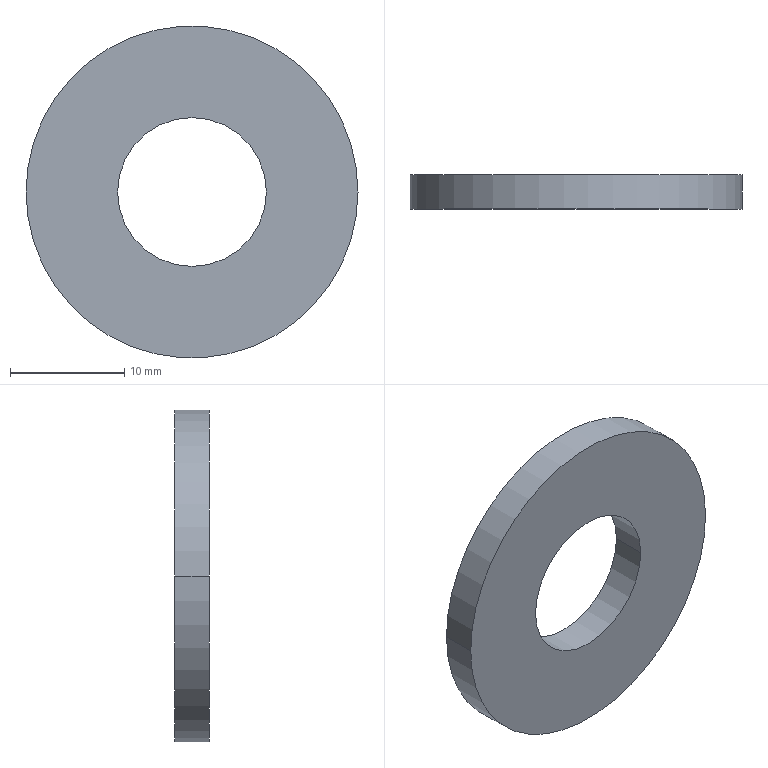Part | STEP file | LIB_29542724_CUP_SPRING_M12 | 1 solid | 6 faces | box 29 x 3 x 29 mm | volume 1583 mm3 | cylinder 4 | plane 2 | commonest cylinder face diameters 13 x2 29 x2
STEP:
#1=CARTESIAN_POINT('',(0.,0.,0.));
#2=DIRECTION('',(0.,0.,1.));
#3=DIRECTION('',(1.,0.,0.));
#4=AXIS2_PLACEMENT_3D('',#1,#2,#3);
#5=CARTESIAN_POINT('',(14.5,0.,0.));
#6=VERTEX_POINT('',#5);
#7=CARTESIAN_POINT('',(-14.5,0.,0.));
#8=VERTEX_POINT('',#7);
#9=CARTESIAN_POINT('',(0.,0.,0.));
#10=DIRECTION('',(0.,1.,0.));
#11=DIRECTION('',(1.,0.,0.));
#12=AXIS2_PLACEMENT_3D('',#9,#10,#11);
#13=CIRCLE('',#12,14.5);
#14=CARTESIAN_POINT('',(0.,0.,0.));
#15=DIRECTION('',(0.,1.,0.));
#16=DIRECTION('',(1.,0.,0.));
#17=AXIS2_PLACEMENT_3D('',#14,#15,#16);
#18=PLANE('',#17);
#19=CARTESIAN_POINT('',(0.,0.));
#20=DIRECTION('',(1.,0.));
#21=AXIS2_PLACEMENT_2D('',#19,#20);
#22=CIRCLE('',#21,14.5);
#23=(GEOMETRIC_REPRESENTATION_CONTEXT(2)PARAMETRIC_REPRESENTATION_CONTEXT()REPRESENTATION_CONTEXT('',''));
#24=DEFINITIONAL_REPRESENTATION('',(#22),#23);
#25=PCURVE('',#18,#24);
#26=CARTESIAN_POINT('',(0.,0.,0.));
#27=DIRECTION('',(0.,1.,0.));
#28=DIRECTION('',(1.,0.,0.));
#29=AXIS2_PLACEMENT_3D('',#26,#27,#28);
#30=CYLINDRICAL_SURFACE('',#29,14.5);
#31=CARTESIAN_POINT('',(0.,0.));
#32=DIRECTION('',(1.,0.));
#33=VECTOR('',#32,1.);
#34=LINE('',#31,#33);
#35=(GEOMETRIC_REPRESENTATION_CONTEXT(2)PARAMETRIC_REPRESENTATION_CONTEXT()REPRESENTATION_CONTEXT('',''));
#36=DEFINITIONAL_REPRESENTATION('',(#34),#35);
#37=PCURVE('',#30,#36);
#38=SURFACE_CURVE('',#13,(#25,#37),.PCURVE_S1.);
#39=EDGE_CURVE('',#6,#8,#38,.T.);
#40=ORIENTED_EDGE('',*,*,#39,.T.);
#41=CARTESIAN_POINT('',(0.,0.,0.));
#42=DIRECTION('',(0.,1.,0.));
#43=DIRECTION('',(-1.,0.,0.));
#44=AXIS2_PLACEMENT_3D('',#41,#42,#43);
#45=CIRCLE('',#44,14.5);
#46=CARTESIAN_POINT('',(0.,0.));
#47=DIRECTION('',(-1.,0.));
#48=AXIS2_PLACEMENT_2D('',#46,#47);
#49=CIRCLE('',#48,14.5);
#50=(GEOMETRIC_REPRESENTATION_CONTEXT(2)PARAMETRIC_REPRESENTATION_CONTEXT()REPRESENTATION_CONTEXT('',''));
#51=DEFINITIONAL_REPRESENTATION('',(#49),#50);
#52=PCURVE('',#18,#51);
#53=CARTESIAN_POINT('',(0.,0.,0.));
#54=DIRECTION('',(0.,1.,0.));
#55=DIRECTION('',(1.,0.,0.));
#56=AXIS2_PLACEMENT_3D('',#53,#54,#55);
#57=CYLINDRICAL_SURFACE('',#56,14.5);
#58=CARTESIAN_POINT('',(3.142,0.));
#59=DIRECTION('',(1.,0.));
#60=VECTOR('',#59,1.);
#61=LINE('',#58,#60);
#62=(GEOMETRIC_REPRESENTATION_CONTEXT(2)PARAMETRIC_REPRESENTATION_CONTEXT()REPRESENTATION_CONTEXT('',''));
#63=DEFINITIONAL_REPRESENTATION('',(#61),#62);
#64=PCURVE('',#57,#63);
#65=SURFACE_CURVE('',#45,(#52,#64),.PCURVE_S1.);
#66=EDGE_CURVE('',#8,#6,#65,.T.);
#67=ORIENTED_EDGE('',*,*,#66,.T.);
#68=EDGE_LOOP('',(#40,#67));
#69=FACE_BOUND('',#68,.F.);
#70=CARTESIAN_POINT('',(6.5,0.,0.));
#71=VERTEX_POINT('',#70);
#72=CARTESIAN_POINT('',(-6.5,0.,0.));
#73=VERTEX_POINT('',#72);
#74=CARTESIAN_POINT('',(0.,0.,0.));
#75=DIRECTION('',(0.,-1.,0.));
#76=DIRECTION('',(1.,0.,0.));
#77=AXIS2_PLACEMENT_3D('',#74,#75,#76);
#78=CIRCLE('',#77,6.5);
#79=CARTESIAN_POINT('',(6.5,0.));
#80=CARTESIAN_POINT('',(6.5,-11.258));
#81=CARTESIAN_POINT('',(-3.25,-5.629));
#82=CARTESIAN_POINT('',(-13.,0.));
#83=CARTESIAN_POINT('',(-3.25,5.629));
#84=CARTESIAN_POINT('',(6.5,11.258));
#85=CARTESIAN_POINT('',(6.5,0.));
#86=(BOUNDED_CURVE()B_SPLINE_CURVE(2,(#79,#80,#81,#82,#83,#84,#85),.UNSPECIFIED.,.T.,.F.)B_SPLINE_CURVE_WITH_KNOTS((1,2,2,2,2,1),(-2.094,0.,2.094,4.189,6.283,8.378),.UNSPECIFIED.)CURVE()GEOMETRIC_REPRESENTATION_ITEM()RATIONAL_B_SPLINE_CURVE((1.,0.5,1.,0.5,1.,0.5,1.))REPRESENTATION_ITEM(''));
#87=(GEOMETRIC_REPRESENTATION_CONTEXT(2)PARAMETRIC_REPRESENTATION_CONTEXT()REPRESENTATION_CONTEXT('',''));
#88=DEFINITIONAL_REPRESENTATION('',(#86),#87);
#89=PCURVE('',#18,#88);
#90=CARTESIAN_POINT('',(0.,0.,0.));
#91=DIRECTION('',(0.,1.,0.));
#92=DIRECTION('',(1.,0.,0.));
#93=AXIS2_PLACEMENT_3D('',#90,#91,#92);
#94=CYLINDRICAL_SURFACE('',#93,6.5);
#95=CARTESIAN_POINT('',(6.283,0.));
#96=DIRECTION('',(-1.,0.));
#97=VECTOR('',#96,1.);
#98=LINE('',#95,#97);
#99=(GEOMETRIC_REPRESENTATION_CONTEXT(2)PARAMETRIC_REPRESENTATION_CONTEXT()REPRESENTATION_CONTEXT('',''));
#100=DEFINITIONAL_REPRESENTATION('',(#98),#99);
#101=PCURVE('',#94,#100);
#102=SURFACE_CURVE('',#78,(#89,#101),.PCURVE_S1.);
#103=EDGE_CURVE('',#71,#73,#102,.T.);
#104=ORIENTED_EDGE('',*,*,#103,.T.);
#105=CARTESIAN_POINT('',(0.,0.,0.));
#106=DIRECTION('',(0.,-1.,0.));
#107=DIRECTION('',(-1.,0.,0.));
#108=AXIS2_PLACEMENT_3D('',#105,#106,#107);
#109=CIRCLE('',#108,6.5);
#110=CARTESIAN_POINT('',(-6.5,0.));
#111=CARTESIAN_POINT('',(-6.5,11.258));
#112=CARTESIAN_POINT('',(3.25,5.629));
#113=CARTESIAN_POINT('',(13.,0.));
#114=CARTESIAN_POINT('',(3.25,-5.629));
#115=CARTESIAN_POINT('',(-6.5,-11.258));
#116=CARTESIAN_POINT('',(-6.5,0.));
#117=(BOUNDED_CURVE()B_SPLINE_CURVE(2,(#110,#111,#112,#113,#114,#115,#116),.UNSPECIFIED.,.T.,.F.)B_SPLINE_CURVE_WITH_KNOTS((1,2,2,2,2,1),(-2.094,0.,2.094,4.189,6.283,8.378),.UNSPECIFIED.)CURVE()GEOMETRIC_REPRESENTATION_ITEM()RATIONAL_B_SPLINE_CURVE((1.,0.5,1.,0.5,1.,0.5,1.))REPRESENTATION_ITEM(''));
#118=(GEOMETRIC_REPRESENTATION_CONTEXT(2)PARAMETRIC_REPRESENTATION_CONTEXT()REPRESENTATION_CONTEXT('',''));
#119=DEFINITIONAL_REPRESENTATION('',(#117),#118);
#120=PCURVE('',#18,#119);
#121=CARTESIAN_POINT('',(0.,0.,0.));
#122=DIRECTION('',(0.,1.,0.));
#123=DIRECTION('',(1.,0.,0.));
#124=AXIS2_PLACEMENT_3D('',#121,#122,#123);
#125=CYLINDRICAL_SURFACE('',#124,6.5);
#126=CARTESIAN_POINT('',(3.142,0.));
#127=DIRECTION('',(-1.,0.));
#128=VECTOR('',#127,1.);
#129=LINE('',#126,#128);
#130=(GEOMETRIC_REPRESENTATION_CONTEXT(2)PARAMETRIC_REPRESENTATION_CONTEXT()REPRESENTATION_CONTEXT('',''));
#131=DEFINITIONAL_REPRESENTATION('',(#129),#130);
#132=PCURVE('',#125,#131);
#133=SURFACE_CURVE('',#109,(#120,#132),.PCURVE_S1.);
#134=EDGE_CURVE('',#73,#71,#133,.T.);
#135=ORIENTED_EDGE('',*,*,#134,.T.);
#136=EDGE_LOOP('',(#104,#135));
#137=FACE_BOUND('',#136,.F.);
#138=ADVANCED_FACE('',(#69,#137),#18,.F.);
#139=CARTESIAN_POINT('',(-14.5,3.,0.));
#140=VERTEX_POINT('',#139);
#141=CARTESIAN_POINT('',(-14.5,0.,0.));
#142=DIRECTION('',(0.,1.,0.));
#143=VECTOR('',#142,1.);
#144=LINE('',#141,#143);
#145=CARTESIAN_POINT('',(3.142,0.));
#146=DIRECTION('',(0.,1.));
#147=VECTOR('',#146,1.);
#148=LINE('',#145,#147);
#149=(GEOMETRIC_REPRESENTATION_CONTEXT(2)PARAMETRIC_REPRESENTATION_CONTEXT()REPRESENTATION_CONTEXT('',''));
#150=DEFINITIONAL_REPRESENTATION('',(#148),#149);
#151=PCURVE('',#30,#150);
#152=CARTESIAN_POINT('',(3.142,0.));
#153=DIRECTION('',(0.,1.));
#154=VECTOR('',#153,1.);
#155=LINE('',#152,#154);
#156=(GEOMETRIC_REPRESENTATION_CONTEXT(2)PARAMETRIC_REPRESENTATION_CONTEXT()REPRESENTATION_CONTEXT('',''));
#157=DEFINITIONAL_REPRESENTATION('',(#155),#156);
#158=PCURVE('',#57,#157);
#159=SURFACE_CURVE('',#144,(#151,#158),.PCURVE_S1.);
#160=EDGE_CURVE('',#8,#140,#159,.T.);
#161=ORIENTED_EDGE('',*,*,#160,.T.);
#162=CARTESIAN_POINT('',(14.5,3.,0.));
#163=VERTEX_POINT('',#162);
#164=CARTESIAN_POINT('',(0.,3.,0.));
#165=DIRECTION('',(0.,1.,0.));
#166=DIRECTION('',(1.,0.,0.));
#167=AXIS2_PLACEMENT_3D('',#164,#165,#166);
#168=CIRCLE('',#167,14.5);
#169=CARTESIAN_POINT('',(0.,3.));
#170=DIRECTION('',(1.,0.));
#171=VECTOR('',#170,1.);
#172=LINE('',#169,#171);
#173=(GEOMETRIC_REPRESENTATION_CONTEXT(2)PARAMETRIC_REPRESENTATION_CONTEXT()REPRESENTATION_CONTEXT('',''));
#174=DEFINITIONAL_REPRESENTATION('',(#172),#173);
#175=PCURVE('',#30,#174);
#176=CARTESIAN_POINT('',(0.,3.,0.));
#177=DIRECTION('',(0.,1.,0.));
#178=DIRECTION('',(1.,0.,0.));
#179=AXIS2_PLACEMENT_3D('',#176,#177,#178);
#180=PLANE('',#179);
#181=CARTESIAN_POINT('',(0.,0.));
#182=DIRECTION('',(1.,0.));
#183=AXIS2_PLACEMENT_2D('',#181,#182);
#184=CIRCLE('',#183,14.5);
#185=(GEOMETRIC_REPRESENTATION_CONTEXT(2)PARAMETRIC_REPRESENTATION_CONTEXT()REPRESENTATION_CONTEXT('',''));
#186=DEFINITIONAL_REPRESENTATION('',(#184),#185);
#187=PCURVE('',#180,#186);
#188=SURFACE_CURVE('',#168,(#175,#187),.PCURVE_S1.);
#189=EDGE_CURVE('',#163,#140,#188,.T.);
#190=ORIENTED_EDGE('',*,*,#189,.F.);
#191=CARTESIAN_POINT('',(14.5,0.,0.));
#192=DIRECTION('',(0.,1.,0.));
#193=VECTOR('',#192,1.);
#194=LINE('',#191,#193);
#195=CARTESIAN_POINT('',(0.,0.));
#196=DIRECTION('',(0.,1.));
#197=VECTOR('',#196,1.);
#198=LINE('',#195,#197);
#199=(GEOMETRIC_REPRESENTATION_CONTEXT(2)PARAMETRIC_REPRESENTATION_CONTEXT()REPRESENTATION_CONTEXT('',''));
#200=DEFINITIONAL_REPRESENTATION('',(#198),#199);
#201=PCURVE('',#30,#200);
#202=CARTESIAN_POINT('',(6.283,0.));
#203=DIRECTION('',(0.,1.));
#204=VECTOR('',#203,1.);
#205=LINE('',#202,#204);
#206=(GEOMETRIC_REPRESENTATION_CONTEXT(2)PARAMETRIC_REPRESENTATION_CONTEXT()REPRESENTATION_CONTEXT('',''));
#207=DEFINITIONAL_REPRESENTATION('',(#205),#206);
#208=PCURVE('',#57,#207);
#209=SURFACE_CURVE('',#194,(#201,#208),.PCURVE_S1.);
#210=EDGE_CURVE('',#6,#163,#209,.T.);
#211=ORIENTED_EDGE('',*,*,#210,.F.);
#212=ORIENTED_EDGE('',*,*,#39,.T.);
#213=EDGE_LOOP('',(#161,#190,#211,#212));
#214=FACE_BOUND('',#213,.T.);
#215=ADVANCED_FACE('',(#214),#30,.T.);
#216=ORIENTED_EDGE('',*,*,#210,.T.);
#217=CARTESIAN_POINT('',(0.,3.,0.));
#218=DIRECTION('',(0.,1.,0.));
#219=DIRECTION('',(-1.,0.,0.));
#220=AXIS2_PLACEMENT_3D('',#217,#218,#219);
#221=CIRCLE('',#220,14.5);
#222=CARTESIAN_POINT('',(3.142,3.));
#223=DIRECTION('',(1.,0.));
#224=VECTOR('',#223,1.);
#225=LINE('',#222,#224);
#226=(GEOMETRIC_REPRESENTATION_CONTEXT(2)PARAMETRIC_REPRESENTATION_CONTEXT()REPRESENTATION_CONTEXT('',''));
#227=DEFINITIONAL_REPRESENTATION('',(#225),#226);
#228=PCURVE('',#57,#227);
#229=CARTESIAN_POINT('',(0.,0.));
#230=DIRECTION('',(-1.,0.));
#231=AXIS2_PLACEMENT_2D('',#229,#230);
#232=CIRCLE('',#231,14.5);
#233=(GEOMETRIC_REPRESENTATION_CONTEXT(2)PARAMETRIC_REPRESENTATION_CONTEXT()REPRESENTATION_CONTEXT('',''));
#234=DEFINITIONAL_REPRESENTATION('',(#232),#233);
#235=PCURVE('',#180,#234);
#236=SURFACE_CURVE('',#221,(#228,#235),.PCURVE_S1.);
#237=EDGE_CURVE('',#140,#163,#236,.T.);
#238=ORIENTED_EDGE('',*,*,#237,.F.);
#239=ORIENTED_EDGE('',*,*,#160,.F.);
#240=ORIENTED_EDGE('',*,*,#66,.T.);
#241=EDGE_LOOP('',(#216,#238,#239,#240));
#242=FACE_BOUND('',#241,.T.);
#243=ADVANCED_FACE('',(#242),#57,.T.);
#244=ORIENTED_EDGE('',*,*,#189,.F.);
#245=ORIENTED_EDGE('',*,*,#237,.F.);
#246=EDGE_LOOP('',(#244,#245));
#247=FACE_BOUND('',#246,.F.);
#248=CARTESIAN_POINT('',(6.5,3.,0.));
#249=VERTEX_POINT('',#248);
#250=CARTESIAN_POINT('',(-6.5,3.,0.));
#251=VERTEX_POINT('',#250);
#252=CARTESIAN_POINT('',(0.,3.,0.));
#253=DIRECTION('',(0.,-1.,0.));
#254=DIRECTION('',(1.,0.,0.));
#255=AXIS2_PLACEMENT_3D('',#252,#253,#254);
#256=CIRCLE('',#255,6.5);
#257=CARTESIAN_POINT('',(6.5,0.));
#258=CARTESIAN_POINT('',(6.5,-11.258));
#259=CARTESIAN_POINT('',(-3.25,-5.629));
#260=CARTESIAN_POINT('',(-13.,0.));
#261=CARTESIAN_POINT('',(-3.25,5.629));
#262=CARTESIAN_POINT('',(6.5,11.258));
#263=CARTESIAN_POINT('',(6.5,0.));
#264=(BOUNDED_CURVE()B_SPLINE_CURVE(2,(#257,#258,#259,#260,#261,#262,#263),.UNSPECIFIED.,.T.,.F.)B_SPLINE_CURVE_WITH_KNOTS((1,2,2,2,2,1),(-2.094,0.,2.094,4.189,6.283,8.378),.UNSPECIFIED.)CURVE()GEOMETRIC_REPRESENTATION_ITEM()RATIONAL_B_SPLINE_CURVE((1.,0.5,1.,0.5,1.,0.5,1.))REPRESENTATION_ITEM(''));
#265=(GEOMETRIC_REPRESENTATION_CONTEXT(2)PARAMETRIC_REPRESENTATION_CONTEXT()REPRESENTATION_CONTEXT('',''));
#266=DEFINITIONAL_REPRESENTATION('',(#264),#265);
#267=PCURVE('',#180,#266);
#268=CARTESIAN_POINT('',(6.283,3.));
#269=DIRECTION('',(-1.,0.));
#270=VECTOR('',#269,1.);
#271=LINE('',#268,#270);
#272=(GEOMETRIC_REPRESENTATION_CONTEXT(2)PARAMETRIC_REPRESENTATION_CONTEXT()REPRESENTATION_CONTEXT('',''));
#273=DEFINITIONAL_REPRESENTATION('',(#271),#272);
#274=PCURVE('',#94,#273);
#275=SURFACE_CURVE('',#256,(#267,#274),.PCURVE_S1.);
#276=EDGE_CURVE('',#249,#251,#275,.T.);
#277=ORIENTED_EDGE('',*,*,#276,.F.);
#278=CARTESIAN_POINT('',(0.,3.,0.));
#279=DIRECTION('',(0.,-1.,0.));
#280=DIRECTION('',(-1.,0.,0.));
#281=AXIS2_PLACEMENT_3D('',#278,#279,#280);
#282=CIRCLE('',#281,6.5);
#283=CARTESIAN_POINT('',(-6.5,0.));
#284=CARTESIAN_POINT('',(-6.5,11.258));
#285=CARTESIAN_POINT('',(3.25,5.629));
#286=CARTESIAN_POINT('',(13.,0.));
#287=CARTESIAN_POINT('',(3.25,-5.629));
#288=CARTESIAN_POINT('',(-6.5,-11.258));
#289=CARTESIAN_POINT('',(-6.5,0.));
#290=(BOUNDED_CURVE()B_SPLINE_CURVE(2,(#283,#284,#285,#286,#287,#288,#289),.UNSPECIFIED.,.T.,.F.)B_SPLINE_CURVE_WITH_KNOTS((1,2,2,2,2,1),(-2.094,0.,2.094,4.189,6.283,8.378),.UNSPECIFIED.)CURVE()GEOMETRIC_REPRESENTATION_ITEM()RATIONAL_B_SPLINE_CURVE((1.,0.5,1.,0.5,1.,0.5,1.))REPRESENTATION_ITEM(''));
#291=(GEOMETRIC_REPRESENTATION_CONTEXT(2)PARAMETRIC_REPRESENTATION_CONTEXT()REPRESENTATION_CONTEXT('',''));
#292=DEFINITIONAL_REPRESENTATION('',(#290),#291);
#293=PCURVE('',#180,#292);
#294=CARTESIAN_POINT('',(3.142,3.));
#295=DIRECTION('',(-1.,0.));
#296=VECTOR('',#295,1.);
#297=LINE('',#294,#296);
#298=(GEOMETRIC_REPRESENTATION_CONTEXT(2)PARAMETRIC_REPRESENTATION_CONTEXT()REPRESENTATION_CONTEXT('',''));
#299=DEFINITIONAL_REPRESENTATION('',(#297),#298);
#300=PCURVE('',#125,#299);
#301=SURFACE_CURVE('',#282,(#293,#300),.PCURVE_S1.);
#302=EDGE_CURVE('',#251,#249,#301,.T.);
#303=ORIENTED_EDGE('',*,*,#302,.F.);
#304=EDGE_LOOP('',(#277,#303));
#305=FACE_BOUND('',#304,.F.);
#306=ADVANCED_FACE('',(#247,#305),#180,.T.);
#307=ORIENTED_EDGE('',*,*,#103,.F.);
#308=CARTESIAN_POINT('',(6.5,0.,0.));
#309=DIRECTION('',(0.,1.,0.));
#310=VECTOR('',#309,1.);
#311=LINE('',#308,#310);
#312=CARTESIAN_POINT('',(6.283,0.));
#313=DIRECTION('',(0.,1.));
#314=VECTOR('',#313,1.);
#315=LINE('',#312,#314);
#316=(GEOMETRIC_REPRESENTATION_CONTEXT(2)PARAMETRIC_REPRESENTATION_CONTEXT()REPRESENTATION_CONTEXT('',''));
#317=DEFINITIONAL_REPRESENTATION('',(#315),#316);
#318=PCURVE('',#94,#317);
#319=CARTESIAN_POINT('',(0.,0.));
#320=DIRECTION('',(0.,1.));
#321=VECTOR('',#320,1.);
#322=LINE('',#319,#321);
#323=(GEOMETRIC_REPRESENTATION_CONTEXT(2)PARAMETRIC_REPRESENTATION_CONTEXT()REPRESENTATION_CONTEXT('',''));
#324=DEFINITIONAL_REPRESENTATION('',(#322),#323);
#325=PCURVE('',#125,#324);
#326=SURFACE_CURVE('',#311,(#318,#325),.PCURVE_S1.);
#327=EDGE_CURVE('',#71,#249,#326,.T.);
#328=ORIENTED_EDGE('',*,*,#327,.T.);
#329=ORIENTED_EDGE('',*,*,#276,.T.);
#330=CARTESIAN_POINT('',(-6.5,0.,0.));
#331=DIRECTION('',(0.,1.,0.));
#332=VECTOR('',#331,1.);
#333=LINE('',#330,#332);
#334=CARTESIAN_POINT('',(3.142,0.));
#335=DIRECTION('',(0.,1.));
#336=VECTOR('',#335,1.);
#337=LINE('',#334,#336);
#338=(GEOMETRIC_REPRESENTATION_CONTEXT(2)PARAMETRIC_REPRESENTATION_CONTEXT()REPRESENTATION_CONTEXT('',''));
#339=DEFINITIONAL_REPRESENTATION('',(#337),#338);
#340=PCURVE('',#94,#339);
#341=CARTESIAN_POINT('',(3.142,0.));
#342=DIRECTION('',(0.,1.));
#343=VECTOR('',#342,1.);
#344=LINE('',#341,#343);
#345=(GEOMETRIC_REPRESENTATION_CONTEXT(2)PARAMETRIC_REPRESENTATION_CONTEXT()REPRESENTATION_CONTEXT('',''));
#346=DEFINITIONAL_REPRESENTATION('',(#344),#345);
#347=PCURVE('',#125,#346);
#348=SURFACE_CURVE('',#333,(#340,#347),.PCURVE_S1.);
#349=EDGE_CURVE('',#73,#251,#348,.T.);
#350=ORIENTED_EDGE('',*,*,#349,.F.);
#351=EDGE_LOOP('',(#307,#328,#329,#350));
#352=FACE_BOUND('',#351,.F.);
#353=ADVANCED_FACE('',(#352),#94,.F.);
#354=ORIENTED_EDGE('',*,*,#134,.F.);
#355=ORIENTED_EDGE('',*,*,#349,.T.);
#356=ORIENTED_EDGE('',*,*,#302,.T.);
#357=ORIENTED_EDGE('',*,*,#327,.F.);
#358=EDGE_LOOP('',(#354,#355,#356,#357));
#359=FACE_BOUND('',#358,.F.);
#360=ADVANCED_FACE('',(#359),#125,.F.);
#361=CLOSED_SHELL('',(#138,#215,#243,#306,#353,#360));
#362=MANIFOLD_SOLID_BREP('',#361);
#363=(LENGTH_UNIT()NAMED_UNIT(*)SI_UNIT(.MILLI.,.METRE.));
#364=UNCERTAINTY_MEASURE_WITH_UNIT(LENGTH_MEASURE(0.0000001),#363,'','');
#365=(NAMED_UNIT(*)PLANE_ANGLE_UNIT()SI_UNIT($,.RADIAN.));
#366=(NAMED_UNIT(*)SI_UNIT($,.STERADIAN.)SOLID_ANGLE_UNIT());
#367=(GEOMETRIC_REPRESENTATION_CONTEXT(3)GLOBAL_UNCERTAINTY_ASSIGNED_CONTEXT((#364))GLOBAL_UNIT_ASSIGNED_CONTEXT((#363,#365,#366))REPRESENTATION_CONTEXT('',''));
#368=ADVANCED_BREP_SHAPE_REPRESENTATION('',(#4,#362),#367);